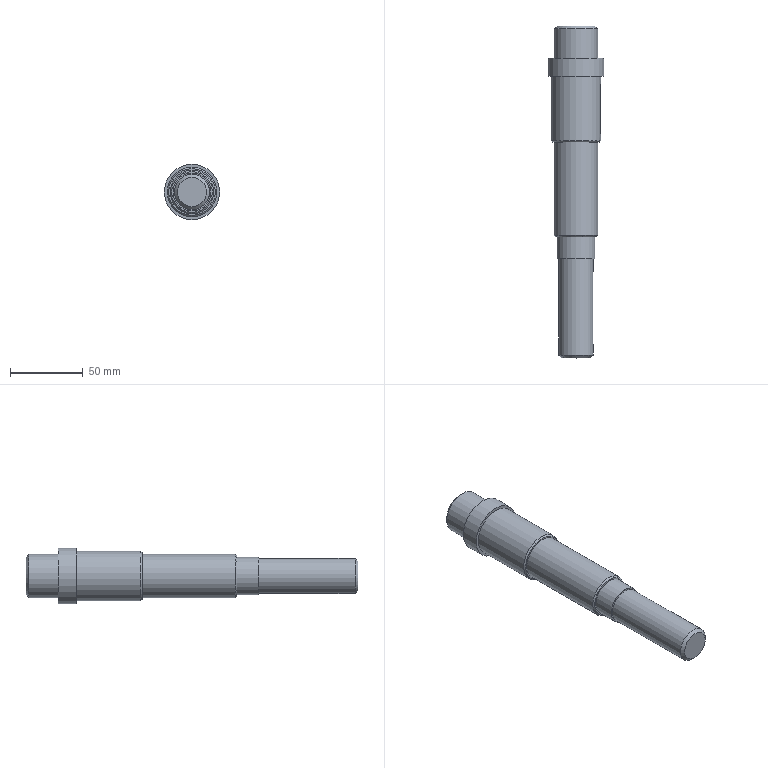Part | NX | features DATUM_CSYS 4, SKETCH 3, CHAMFER 2, DATUM_PLANE 2, EXTRUDE 2, CPROJ 1, SWP104 1 | 1 solid | 27 faces | box 38 x 227.5 x 38 mm | volume 152701 mm3 | plane 13 | cylinder 10 | cone 4 | commonest cylinder face diameters 6 x2 8 x2 30 x2 24 x1 26 x1 34 x1
STEP:
#1=CARTESIAN_POINT('',(0.,227.5,-13.));
#2=VERTEX_POINT('',#1);
#3=CARTESIAN_POINT('',(0.,227.5,0.));
#4=DIRECTION('',(0.,-1.,0.));
#5=DIRECTION('',(0.,0.,-1.));
#6=AXIS2_PLACEMENT_3D('',#3,#4,#5);
#7=CIRCLE('',#6,13.);
#8=EDGE_CURVE('',#2,#2,#7,.F.);
#9=ORIENTED_EDGE('',*,*,#8,.T.);
#10=EDGE_LOOP('',(#9));
#11=FACE_BOUND('',#10,.T.);
#12=CARTESIAN_POINT('',(0.,227.5,0.));
#13=DIRECTION('',(0.,-1.,0.));
#14=DIRECTION('',(0.,0.,-1.));
#15=AXIS2_PLACEMENT_3D('',#12,#13,#14);
#16=PLANE('',#15);
#17=ADVANCED_FACE('',(#11),#16,.F.);
#18=CARTESIAN_POINT('',(0.,225.5,-15.));
#19=VERTEX_POINT('',#18);
#20=CARTESIAN_POINT('',(0.,225.5,0.));
#21=DIRECTION('',(0.,-1.,0.));
#22=DIRECTION('',(0.,0.,-1.));
#23=AXIS2_PLACEMENT_3D('',#20,#21,#22);
#24=CIRCLE('',#23,15.);
#25=EDGE_CURVE('',#19,#19,#24,.T.);
#26=ORIENTED_EDGE('',*,*,#25,.T.);
#27=EDGE_LOOP('',(#26));
#28=FACE_BOUND('',#27,.T.);
#29=CARTESIAN_POINT('',(0.,205.5,-15.));
#30=VERTEX_POINT('',#29);
#31=CARTESIAN_POINT('',(0.,205.5,0.));
#32=DIRECTION('',(0.,-1.,0.));
#33=DIRECTION('',(0.,0.,-1.));
#34=AXIS2_PLACEMENT_3D('',#31,#32,#33);
#35=CIRCLE('',#34,15.);
#36=EDGE_CURVE('',#30,#30,#35,.T.);
#37=ORIENTED_EDGE('',*,*,#36,.F.);
#38=EDGE_LOOP('',(#37));
#39=FACE_BOUND('',#38,.T.);
#40=CARTESIAN_POINT('',(0.,227.5,0.));
#41=DIRECTION('',(0.,-1.,0.));
#42=DIRECTION('',(0.,0.,-1.));
#43=AXIS2_PLACEMENT_3D('',#40,#41,#42);
#44=CYLINDRICAL_SURFACE('',#43,15.);
#45=ADVANCED_FACE('',(#28,#39),#44,.T.);
#46=CARTESIAN_POINT('',(0.,205.5,-19.));
#47=VERTEX_POINT('',#46);
#48=CARTESIAN_POINT('',(0.,205.5,0.));
#49=DIRECTION('',(0.,-1.,0.));
#50=DIRECTION('',(0.,0.,-1.));
#51=AXIS2_PLACEMENT_3D('',#48,#49,#50);
#52=CIRCLE('',#51,19.);
#53=EDGE_CURVE('',#47,#47,#52,.T.);
#54=ORIENTED_EDGE('',*,*,#53,.F.);
#55=EDGE_LOOP('',(#54));
#56=FACE_BOUND('',#55,.T.);
#57=ORIENTED_EDGE('',*,*,#36,.T.);
#58=EDGE_LOOP('',(#57));
#59=FACE_BOUND('',#58,.T.);
#60=CARTESIAN_POINT('',(0.,205.5,15.));
#61=DIRECTION('',(0.,-1.,0.));
#62=DIRECTION('',(0.,0.,-1.));
#63=AXIS2_PLACEMENT_3D('',#60,#61,#62);
#64=PLANE('',#63);
#65=ADVANCED_FACE('',(#56,#59),#64,.F.);
#66=CARTESIAN_POINT('',(0.,193.,-19.));
#67=VERTEX_POINT('',#66);
#68=CARTESIAN_POINT('',(0.,193.,0.));
#69=DIRECTION('',(0.,-1.,0.));
#70=DIRECTION('',(0.,0.,-1.));
#71=AXIS2_PLACEMENT_3D('',#68,#69,#70);
#72=CIRCLE('',#71,19.);
#73=EDGE_CURVE('',#67,#67,#72,.T.);
#74=ORIENTED_EDGE('',*,*,#73,.F.);
#75=EDGE_LOOP('',(#74));
#76=FACE_BOUND('',#75,.T.);
#77=ORIENTED_EDGE('',*,*,#53,.T.);
#78=EDGE_LOOP('',(#77));
#79=FACE_BOUND('',#78,.T.);
#80=CARTESIAN_POINT('',(0.,227.5,0.));
#81=DIRECTION('',(0.,-1.,0.));
#82=DIRECTION('',(0.,0.,-1.));
#83=AXIS2_PLACEMENT_3D('',#80,#81,#82);
#84=CYLINDRICAL_SURFACE('',#83,19.);
#85=ADVANCED_FACE('',(#76,#79),#84,.T.);
#86=CARTESIAN_POINT('',(0.,193.,-17.));
#87=VERTEX_POINT('',#86);
#88=CARTESIAN_POINT('',(0.,193.,0.));
#89=DIRECTION('',(0.,-1.,0.));
#90=DIRECTION('',(0.,0.,-1.));
#91=AXIS2_PLACEMENT_3D('',#88,#89,#90);
#92=CIRCLE('',#91,17.);
#93=EDGE_CURVE('',#87,#87,#92,.T.);
#94=ORIENTED_EDGE('',*,*,#93,.F.);
#95=EDGE_LOOP('',(#94));
#96=FACE_BOUND('',#95,.T.);
#97=ORIENTED_EDGE('',*,*,#73,.T.);
#98=EDGE_LOOP('',(#97));
#99=FACE_BOUND('',#98,.T.);
#100=CARTESIAN_POINT('',(0.,193.,19.));
#101=DIRECTION('',(0.,1.,0.));
#102=DIRECTION('',(0.,0.,1.));
#103=AXIS2_PLACEMENT_3D('',#100,#101,#102);
#104=PLANE('',#103);
#105=ADVANCED_FACE('',(#96,#99),#104,.F.);
#106=CARTESIAN_POINT('',(16.523,156.5,4.));
#107=VERTEX_POINT('',#106);
#108=CARTESIAN_POINT('',(16.523,184.5,4.));
#109=VERTEX_POINT('',#108);
#110=CARTESIAN_POINT('',(16.523,227.5,4.));
#111=DIRECTION('',(0.,-1.,0.));
#112=VECTOR('',#111,1000.);
#113=LINE('',#110,#112);
#114=EDGE_CURVE('',#107,#109,#113,.F.);
#115=ORIENTED_EDGE('',*,*,#114,.T.);
#116=CARTESIAN_POINT('',(16.523,184.5,-4.));
#117=VERTEX_POINT('',#116);
#118=CARTESIAN_POINT('',(16.523,184.5,4.));
#119=CARTESIAN_POINT('',(16.523,185.561,4.));
#120=CARTESIAN_POINT('',(16.765,187.627,3.133));
#121=CARTESIAN_POINT('',(17.118,188.936,0.005404));
#122=CARTESIAN_POINT('',(16.765,187.629,-3.134));
#123=CARTESIAN_POINT('',(16.523,185.561,-4.));
#124=CARTESIAN_POINT('',(16.523,184.5,-4.));
#125=B_SPLINE_CURVE_WITH_KNOTS('',3,(#118,#119,#120,#121,#122,#123,#124),.UNSPECIFIED.,.F.,.F.,(4,1,1,1,4),(0.,0.003137,0.006273,0.00941,0.01255),.UNSPECIFIED.);
#126=EDGE_CURVE('',#109,#117,#125,.T.);
#127=ORIENTED_EDGE('',*,*,#126,.T.);
#128=CARTESIAN_POINT('',(16.523,156.5,-4.));
#129=VERTEX_POINT('',#128);
#130=CARTESIAN_POINT('',(16.523,227.5,-4.));
#131=DIRECTION('',(0.,-1.,0.));
#132=VECTOR('',#131,1000.);
#133=LINE('',#130,#132);
#134=EDGE_CURVE('',#117,#129,#133,.T.);
#135=ORIENTED_EDGE('',*,*,#134,.T.);
#136=CARTESIAN_POINT('',(16.523,156.5,-4.));
#137=CARTESIAN_POINT('',(16.523,155.439,-4.));
#138=CARTESIAN_POINT('',(16.765,153.373,-3.133));
#139=CARTESIAN_POINT('',(17.118,152.064,-0.005404));
#140=CARTESIAN_POINT('',(16.765,153.371,3.134));
#141=CARTESIAN_POINT('',(16.523,155.439,4.));
#142=CARTESIAN_POINT('',(16.523,156.5,4.));
#143=B_SPLINE_CURVE_WITH_KNOTS('',3,(#136,#137,#138,#139,#140,#141,#142),.UNSPECIFIED.,.F.,.F.,(4,1,1,1,4),(0.,0.003137,0.006273,0.00941,0.01255),.UNSPECIFIED.);
#144=EDGE_CURVE('',#129,#107,#143,.T.);
#145=ORIENTED_EDGE('',*,*,#144,.T.);
#146=EDGE_LOOP('',(#115,#127,#135,#145));
#147=FACE_BOUND('',#146,.T.);
#148=CARTESIAN_POINT('',(0.,149.,17.));
#149=VERTEX_POINT('',#148);
#150=CARTESIAN_POINT('',(0.,149.,0.));
#151=DIRECTION('',(0.,1.,0.));
#152=DIRECTION('',(0.,0.,1.));
#153=AXIS2_PLACEMENT_3D('',#150,#151,#152);
#154=CIRCLE('',#153,17.);
#155=EDGE_CURVE('',#149,#149,#154,.T.);
#156=ORIENTED_EDGE('',*,*,#155,.T.);
#157=EDGE_LOOP('',(#156));
#158=FACE_BOUND('',#157,.T.);
#159=ORIENTED_EDGE('',*,*,#93,.T.);
#160=EDGE_LOOP('',(#159));
#161=FACE_BOUND('',#160,.T.);
#162=CARTESIAN_POINT('',(0.,227.5,0.));
#163=DIRECTION('',(0.,-1.,0.));
#164=DIRECTION('',(0.,0.,-1.));
#165=AXIS2_PLACEMENT_3D('',#162,#163,#164);
#166=CYLINDRICAL_SURFACE('',#165,17.);
#167=ADVANCED_FACE('',(#147,#158,#161),#166,.T.);
#168=CARTESIAN_POINT('',(0.,148.,16.));
#169=VERTEX_POINT('',#168);
#170=CARTESIAN_POINT('',(0.,148.,0.));
#171=DIRECTION('',(0.,1.,0.));
#172=DIRECTION('',(0.,0.,1.));
#173=AXIS2_PLACEMENT_3D('',#170,#171,#172);
#174=CIRCLE('',#173,16.);
#175=EDGE_CURVE('',#169,#169,#174,.F.);
#176=ORIENTED_EDGE('',*,*,#175,.T.);
#177=EDGE_LOOP('',(#176));
#178=FACE_BOUND('',#177,.T.);
#179=CARTESIAN_POINT('',(0.,148.,-15.));
#180=VERTEX_POINT('',#179);
#181=CARTESIAN_POINT('',(0.,148.,0.));
#182=DIRECTION('',(0.,-1.,0.));
#183=DIRECTION('',(0.,0.,-1.));
#184=AXIS2_PLACEMENT_3D('',#181,#182,#183);
#185=CIRCLE('',#184,15.);
#186=EDGE_CURVE('',#180,#180,#185,.T.);
#187=ORIENTED_EDGE('',*,*,#186,.F.);
#188=EDGE_LOOP('',(#187));
#189=FACE_BOUND('',#188,.T.);
#190=CARTESIAN_POINT('',(0.,148.,17.));
#191=DIRECTION('',(0.,1.,0.));
#192=DIRECTION('',(0.,0.,1.));
#193=AXIS2_PLACEMENT_3D('',#190,#191,#192);
#194=PLANE('',#193);
#195=ADVANCED_FACE('',(#178,#189),#194,.F.);
#196=CARTESIAN_POINT('',(0.,84.,15.));
#197=VERTEX_POINT('',#196);
#198=CARTESIAN_POINT('',(0.,84.,0.));
#199=DIRECTION('',(0.,1.,0.));
#200=DIRECTION('',(0.,0.,1.));
#201=AXIS2_PLACEMENT_3D('',#198,#199,#200);
#202=CIRCLE('',#201,15.);
#203=EDGE_CURVE('',#197,#197,#202,.T.);
#204=ORIENTED_EDGE('',*,*,#203,.T.);
#205=EDGE_LOOP('',(#204));
#206=FACE_BOUND('',#205,.T.);
#207=ORIENTED_EDGE('',*,*,#186,.T.);
#208=EDGE_LOOP('',(#207));
#209=FACE_BOUND('',#208,.T.);
#210=CARTESIAN_POINT('',(0.,227.5,0.));
#211=DIRECTION('',(0.,-1.,0.));
#212=DIRECTION('',(0.,0.,-1.));
#213=AXIS2_PLACEMENT_3D('',#210,#211,#212);
#214=CYLINDRICAL_SURFACE('',#213,15.);
#215=ADVANCED_FACE('',(#206,#209),#214,.T.);
#216=CARTESIAN_POINT('',(0.,83.,14.));
#217=VERTEX_POINT('',#216);
#218=CARTESIAN_POINT('',(0.,83.,0.));
#219=DIRECTION('',(0.,1.,0.));
#220=DIRECTION('',(0.,0.,1.));
#221=AXIS2_PLACEMENT_3D('',#218,#219,#220);
#222=CIRCLE('',#221,14.);
#223=EDGE_CURVE('',#217,#217,#222,.F.);
#224=ORIENTED_EDGE('',*,*,#223,.T.);
#225=EDGE_LOOP('',(#224));
#226=FACE_BOUND('',#225,.T.);
#227=CARTESIAN_POINT('',(0.,83.,-13.));
#228=VERTEX_POINT('',#227);
#229=CARTESIAN_POINT('',(0.,83.,0.));
#230=DIRECTION('',(0.,-1.,0.));
#231=DIRECTION('',(0.,0.,-1.));
#232=AXIS2_PLACEMENT_3D('',#229,#230,#231);
#233=CIRCLE('',#232,13.);
#234=EDGE_CURVE('',#228,#228,#233,.T.);
#235=ORIENTED_EDGE('',*,*,#234,.F.);
#236=EDGE_LOOP('',(#235));
#237=FACE_BOUND('',#236,.T.);
#238=CARTESIAN_POINT('',(0.,83.,15.));
#239=DIRECTION('',(0.,1.,0.));
#240=DIRECTION('',(0.,0.,1.));
#241=AXIS2_PLACEMENT_3D('',#238,#239,#240);
#242=PLANE('',#241);
#243=ADVANCED_FACE('',(#226,#237),#242,.F.);
#244=CARTESIAN_POINT('',(0.,68.,-13.));
#245=VERTEX_POINT('',#244);
#246=CARTESIAN_POINT('',(0.,68.,0.));
#247=DIRECTION('',(0.,-1.,0.));
#248=DIRECTION('',(0.,0.,-1.));
#249=AXIS2_PLACEMENT_3D('',#246,#247,#248);
#250=CIRCLE('',#249,13.);
#251=EDGE_CURVE('',#245,#245,#250,.T.);
#252=ORIENTED_EDGE('',*,*,#251,.F.);
#253=EDGE_LOOP('',(#252));
#254=FACE_BOUND('',#253,.T.);
#255=ORIENTED_EDGE('',*,*,#234,.T.);
#256=EDGE_LOOP('',(#255));
#257=FACE_BOUND('',#256,.T.);
#258=CARTESIAN_POINT('',(0.,227.5,0.));
#259=DIRECTION('',(0.,-1.,0.));
#260=DIRECTION('',(0.,0.,-1.));
#261=AXIS2_PLACEMENT_3D('',#258,#259,#260);
#262=CYLINDRICAL_SURFACE('',#261,13.);
#263=ADVANCED_FACE('',(#254,#257),#262,.T.);
#264=CARTESIAN_POINT('',(0.,68.,-12.));
#265=VERTEX_POINT('',#264);
#266=CARTESIAN_POINT('',(0.,68.,0.));
#267=DIRECTION('',(0.,-1.,0.));
#268=DIRECTION('',(0.,0.,-1.));
#269=AXIS2_PLACEMENT_3D('',#266,#267,#268);
#270=CIRCLE('',#269,12.);
#271=EDGE_CURVE('',#265,#265,#270,.T.);
#272=ORIENTED_EDGE('',*,*,#271,.F.);
#273=EDGE_LOOP('',(#272));
#274=FACE_BOUND('',#273,.T.);
#275=ORIENTED_EDGE('',*,*,#251,.T.);
#276=EDGE_LOOP('',(#275));
#277=FACE_BOUND('',#276,.T.);
#278=CARTESIAN_POINT('',(0.,68.,13.));
#279=DIRECTION('',(0.,1.,0.));
#280=DIRECTION('',(0.,0.,1.));
#281=AXIS2_PLACEMENT_3D('',#278,#279,#280);
#282=PLANE('',#281);
#283=ADVANCED_FACE('',(#274,#277),#282,.F.);
#284=CARTESIAN_POINT('',(11.619,10.,3.));
#285=VERTEX_POINT('',#284);
#286=CARTESIAN_POINT('',(11.619,58.,3.));
#287=VERTEX_POINT('',#286);
#288=CARTESIAN_POINT('',(11.619,227.5,3.));
#289=DIRECTION('',(0.,-1.,0.));
#290=VECTOR('',#289,1000.);
#291=LINE('',#288,#290);
#292=EDGE_CURVE('',#285,#287,#291,.F.);
#293=ORIENTED_EDGE('',*,*,#292,.T.);
#294=CARTESIAN_POINT('',(11.619,58.,-3.));
#295=VERTEX_POINT('',#294);
#296=CARTESIAN_POINT('',(11.619,58.,3.));
#297=CARTESIAN_POINT('',(11.619,58.796,3.));
#298=CARTESIAN_POINT('',(11.813,60.345,2.35));
#299=CARTESIAN_POINT('',(12.094,61.327,0.004206));
#300=CARTESIAN_POINT('',(11.813,60.346,-2.35));
#301=CARTESIAN_POINT('',(11.619,58.796,-3.));
#302=CARTESIAN_POINT('',(11.619,58.,-3.));
#303=B_SPLINE_CURVE_WITH_KNOTS('',3,(#296,#297,#298,#299,#300,#301,#302),.UNSPECIFIED.,.F.,.F.,(4,1,1,1,4),(0.,0.002353,0.004707,0.00706,0.009414),.UNSPECIFIED.);
#304=EDGE_CURVE('',#287,#295,#303,.T.);
#305=ORIENTED_EDGE('',*,*,#304,.T.);
#306=CARTESIAN_POINT('',(11.619,10.,-3.));
#307=VERTEX_POINT('',#306);
#308=CARTESIAN_POINT('',(11.619,227.5,-3.));
#309=DIRECTION('',(0.,-1.,0.));
#310=VECTOR('',#309,1000.);
#311=LINE('',#308,#310);
#312=EDGE_CURVE('',#295,#307,#311,.T.);
#313=ORIENTED_EDGE('',*,*,#312,.T.);
#314=CARTESIAN_POINT('',(11.619,10.,-3.));
#315=CARTESIAN_POINT('',(11.619,9.204,-3.));
#316=CARTESIAN_POINT('',(11.813,7.655,-2.35));
#317=CARTESIAN_POINT('',(12.094,6.673,-0.004206));
#318=CARTESIAN_POINT('',(11.813,7.654,2.35));
#319=CARTESIAN_POINT('',(11.619,9.204,3.));
#320=CARTESIAN_POINT('',(11.619,10.,3.));
#321=B_SPLINE_CURVE_WITH_KNOTS('',3,(#314,#315,#316,#317,#318,#319,#320),.UNSPECIFIED.,.F.,.F.,(4,1,1,1,4),(0.,0.002353,0.004707,0.00706,0.009414),.UNSPECIFIED.);
#322=EDGE_CURVE('',#307,#285,#321,.T.);
#323=ORIENTED_EDGE('',*,*,#322,.T.);
#324=EDGE_LOOP('',(#293,#305,#313,#323));
#325=FACE_BOUND('',#324,.T.);
#326=CARTESIAN_POINT('',(0.,2.,12.));
#327=VERTEX_POINT('',#326);
#328=CARTESIAN_POINT('',(0.,2.,0.));
#329=DIRECTION('',(0.,1.,0.));
#330=DIRECTION('',(0.,0.,1.));
#331=AXIS2_PLACEMENT_3D('',#328,#329,#330);
#332=CIRCLE('',#331,12.);
#333=EDGE_CURVE('',#327,#327,#332,.T.);
#334=ORIENTED_EDGE('',*,*,#333,.T.);
#335=EDGE_LOOP('',(#334));
#336=FACE_BOUND('',#335,.T.);
#337=ORIENTED_EDGE('',*,*,#271,.T.);
#338=EDGE_LOOP('',(#337));
#339=FACE_BOUND('',#338,.T.);
#340=CARTESIAN_POINT('',(0.,227.5,0.));
#341=DIRECTION('',(0.,-1.,0.));
#342=DIRECTION('',(0.,0.,-1.));
#343=AXIS2_PLACEMENT_3D('',#340,#341,#342);
#344=CYLINDRICAL_SURFACE('',#343,12.);
#345=ADVANCED_FACE('',(#325,#336,#339),#344,.T.);
#346=CARTESIAN_POINT('',(0.,0.,10.));
#347=VERTEX_POINT('',#346);
#348=CARTESIAN_POINT('',(0.,0.,0.));
#349=DIRECTION('',(0.,1.,0.));
#350=DIRECTION('',(0.,0.,1.));
#351=AXIS2_PLACEMENT_3D('',#348,#349,#350);
#352=CIRCLE('',#351,10.);
#353=EDGE_CURVE('',#347,#347,#352,.F.);
#354=ORIENTED_EDGE('',*,*,#353,.T.);
#355=EDGE_LOOP('',(#354));
#356=FACE_BOUND('',#355,.T.);
#357=CARTESIAN_POINT('',(0.,0.,12.));
#358=DIRECTION('',(0.,1.,0.));
#359=DIRECTION('',(0.,0.,1.));
#360=AXIS2_PLACEMENT_3D('',#357,#358,#359);
#361=PLANE('',#360);
#362=ADVANCED_FACE('',(#356),#361,.F.);
#363=ORIENTED_EDGE('',*,*,#333,.F.);
#364=EDGE_LOOP('',(#363));
#365=FACE_BOUND('',#364,.T.);
#366=ORIENTED_EDGE('',*,*,#353,.F.);
#367=EDGE_LOOP('',(#366));
#368=FACE_BOUND('',#367,.T.);
#369=CARTESIAN_POINT('',(0.,0.,0.));
#370=DIRECTION('',(0.,1.,0.));
#371=DIRECTION('',(0.,0.,1.));
#372=AXIS2_PLACEMENT_3D('',#369,#370,#371);
#373=CONICAL_SURFACE('',#372,10.,0.7854);
#374=ADVANCED_FACE('',(#365,#368),#373,.T.);
#375=ORIENTED_EDGE('',*,*,#8,.F.);
#376=EDGE_LOOP('',(#375));
#377=FACE_BOUND('',#376,.T.);
#378=ORIENTED_EDGE('',*,*,#25,.F.);
#379=EDGE_LOOP('',(#378));
#380=FACE_BOUND('',#379,.T.);
#381=CARTESIAN_POINT('',(0.,225.5,0.));
#382=DIRECTION('',(0.,-1.,0.));
#383=DIRECTION('',(0.,0.,-1.));
#384=AXIS2_PLACEMENT_3D('',#381,#382,#383);
#385=CONICAL_SURFACE('',#384,15.,0.7854);
#386=ADVANCED_FACE('',(#377,#380),#385,.T.);
#387=ORIENTED_EDGE('',*,*,#203,.F.);
#388=EDGE_LOOP('',(#387));
#389=FACE_BOUND('',#388,.T.);
#390=ORIENTED_EDGE('',*,*,#223,.F.);
#391=EDGE_LOOP('',(#390));
#392=FACE_BOUND('',#391,.T.);
#393=CARTESIAN_POINT('',(0.,83.,0.));
#394=DIRECTION('',(0.,1.,0.));
#395=DIRECTION('',(0.,0.,1.));
#396=AXIS2_PLACEMENT_3D('',#393,#394,#395);
#397=CONICAL_SURFACE('',#396,14.,0.7854);
#398=ADVANCED_FACE('',(#389,#392),#397,.T.);
#399=ORIENTED_EDGE('',*,*,#155,.F.);
#400=EDGE_LOOP('',(#399));
#401=FACE_BOUND('',#400,.T.);
#402=ORIENTED_EDGE('',*,*,#175,.F.);
#403=EDGE_LOOP('',(#402));
#404=FACE_BOUND('',#403,.T.);
#405=CARTESIAN_POINT('',(0.,148.,0.));
#406=DIRECTION('',(0.,1.,0.));
#407=DIRECTION('',(0.,0.,1.));
#408=AXIS2_PLACEMENT_3D('',#405,#406,#407);
#409=CONICAL_SURFACE('',#408,16.,0.7854);
#410=ADVANCED_FACE('',(#401,#404),#409,.T.);
#411=CARTESIAN_POINT('',(12.5,156.5,-4.));
#412=VERTEX_POINT('',#411);
#413=CARTESIAN_POINT('',(12.5,156.5,-4.));
#414=DIRECTION('',(1.,0.,0.));
#415=VECTOR('',#414,1000.);
#416=LINE('',#413,#415);
#417=EDGE_CURVE('',#129,#412,#416,.F.);
#418=ORIENTED_EDGE('',*,*,#417,.T.);
#419=CARTESIAN_POINT('',(12.5,156.5,4.));
#420=VERTEX_POINT('',#419);
#421=CARTESIAN_POINT('',(12.5,156.5,0.));
#422=DIRECTION('',(1.,0.,0.));
#423=DIRECTION('',(0.,1.,0.));
#424=AXIS2_PLACEMENT_3D('',#421,#422,#423);
#425=CIRCLE('',#424,4.);
#426=EDGE_CURVE('',#412,#420,#425,.F.);
#427=ORIENTED_EDGE('',*,*,#426,.T.);
#428=CARTESIAN_POINT('',(12.5,156.5,4.));
#429=DIRECTION('',(1.,0.,0.));
#430=VECTOR('',#429,1000.);
#431=LINE('',#428,#430);
#432=EDGE_CURVE('',#107,#420,#431,.F.);
#433=ORIENTED_EDGE('',*,*,#432,.F.);
#434=ORIENTED_EDGE('',*,*,#144,.F.);
#435=EDGE_LOOP('',(#418,#427,#433,#434));
#436=FACE_BOUND('',#435,.T.);
#437=CARTESIAN_POINT('',(12.5,156.5,0.));
#438=DIRECTION('',(1.,0.,0.));
#439=DIRECTION('',(0.,0.,-1.));
#440=AXIS2_PLACEMENT_3D('',#437,#438,#439);
#441=CYLINDRICAL_SURFACE('',#440,4.);
#442=ADVANCED_FACE('',(#436),#441,.F.);
#443=CARTESIAN_POINT('',(12.5,184.5,-4.));
#444=VERTEX_POINT('',#443);
#445=CARTESIAN_POINT('',(12.5,184.5,-4.));
#446=DIRECTION('',(1.,0.,0.));
#447=VECTOR('',#446,1000.);
#448=LINE('',#445,#447);
#449=EDGE_CURVE('',#117,#444,#448,.F.);
#450=ORIENTED_EDGE('',*,*,#449,.T.);
#451=CARTESIAN_POINT('',(12.5,156.5,-4.));
#452=DIRECTION('',(0.,1.,0.));
#453=VECTOR('',#452,1000.);
#454=LINE('',#451,#453);
#455=EDGE_CURVE('',#444,#412,#454,.F.);
#456=ORIENTED_EDGE('',*,*,#455,.T.);
#457=ORIENTED_EDGE('',*,*,#417,.F.);
#458=ORIENTED_EDGE('',*,*,#134,.F.);
#459=EDGE_LOOP('',(#450,#456,#457,#458));
#460=FACE_BOUND('',#459,.T.);
#461=CARTESIAN_POINT('',(12.5,156.5,-4.));
#462=DIRECTION('',(0.,0.,-1.));
#463=DIRECTION('',(0.,1.,0.));
#464=AXIS2_PLACEMENT_3D('',#461,#462,#463);
#465=PLANE('',#464);
#466=ADVANCED_FACE('',(#460),#465,.F.);
#467=CARTESIAN_POINT('',(12.5,184.5,4.));
#468=VERTEX_POINT('',#467);
#469=CARTESIAN_POINT('',(12.5,184.5,4.));
#470=DIRECTION('',(1.,0.,0.));
#471=VECTOR('',#470,1000.);
#472=LINE('',#469,#471);
#473=EDGE_CURVE('',#109,#468,#472,.F.);
#474=ORIENTED_EDGE('',*,*,#473,.T.);
#475=CARTESIAN_POINT('',(12.5,184.5,0.));
#476=DIRECTION('',(1.,0.,0.));
#477=DIRECTION('',(0.,1.,0.));
#478=AXIS2_PLACEMENT_3D('',#475,#476,#477);
#479=CIRCLE('',#478,4.);
#480=EDGE_CURVE('',#468,#444,#479,.F.);
#481=ORIENTED_EDGE('',*,*,#480,.T.);
#482=ORIENTED_EDGE('',*,*,#449,.F.);
#483=ORIENTED_EDGE('',*,*,#126,.F.);
#484=EDGE_LOOP('',(#474,#481,#482,#483));
#485=FACE_BOUND('',#484,.T.);
#486=CARTESIAN_POINT('',(12.5,184.5,0.));
#487=DIRECTION('',(1.,0.,0.));
#488=DIRECTION('',(0.,0.,-1.));
#489=AXIS2_PLACEMENT_3D('',#486,#487,#488);
#490=CYLINDRICAL_SURFACE('',#489,4.);
#491=ADVANCED_FACE('',(#485),#490,.F.);
#492=ORIENTED_EDGE('',*,*,#432,.T.);
#493=CARTESIAN_POINT('',(12.5,184.5,4.));
#494=DIRECTION('',(0.,-1.,0.));
#495=VECTOR('',#494,1000.);
#496=LINE('',#493,#495);
#497=EDGE_CURVE('',#420,#468,#496,.F.);
#498=ORIENTED_EDGE('',*,*,#497,.T.);
#499=ORIENTED_EDGE('',*,*,#473,.F.);
#500=ORIENTED_EDGE('',*,*,#114,.F.);
#501=EDGE_LOOP('',(#492,#498,#499,#500));
#502=FACE_BOUND('',#501,.T.);
#503=CARTESIAN_POINT('',(12.5,184.5,4.));
#504=DIRECTION('',(0.,0.,1.));
#505=DIRECTION('',(0.,-1.,0.));
#506=AXIS2_PLACEMENT_3D('',#503,#504,#505);
#507=PLANE('',#506);
#508=ADVANCED_FACE('',(#502),#507,.F.);
#509=ORIENTED_EDGE('',*,*,#426,.F.);
#510=ORIENTED_EDGE('',*,*,#455,.F.);
#511=ORIENTED_EDGE('',*,*,#480,.F.);
#512=ORIENTED_EDGE('',*,*,#497,.F.);
#513=EDGE_LOOP('',(#509,#510,#511,#512));
#514=FACE_BOUND('',#513,.T.);
#515=CARTESIAN_POINT('',(12.5,156.5,0.));
#516=DIRECTION('',(1.,0.,0.));
#517=DIRECTION('',(0.,0.,-1.));
#518=AXIS2_PLACEMENT_3D('',#515,#516,#517);
#519=PLANE('',#518);
#520=ADVANCED_FACE('',(#514),#519,.T.);
#521=CARTESIAN_POINT('',(8.9,10.,-3.));
#522=VERTEX_POINT('',#521);
#523=CARTESIAN_POINT('',(8.9,10.,-3.));
#524=DIRECTION('',(1.,0.,0.));
#525=VECTOR('',#524,1000.);
#526=LINE('',#523,#525);
#527=EDGE_CURVE('',#307,#522,#526,.F.);
#528=ORIENTED_EDGE('',*,*,#527,.T.);
#529=CARTESIAN_POINT('',(8.9,10.,3.));
#530=VERTEX_POINT('',#529);
#531=CARTESIAN_POINT('',(8.9,10.,0.));
#532=DIRECTION('',(1.,0.,0.));
#533=DIRECTION('',(0.,1.,0.));
#534=AXIS2_PLACEMENT_3D('',#531,#532,#533);
#535=CIRCLE('',#534,3.);
#536=EDGE_CURVE('',#522,#530,#535,.F.);
#537=ORIENTED_EDGE('',*,*,#536,.T.);
#538=CARTESIAN_POINT('',(8.9,10.,3.));
#539=DIRECTION('',(1.,0.,0.));
#540=VECTOR('',#539,1000.);
#541=LINE('',#538,#540);
#542=EDGE_CURVE('',#285,#530,#541,.F.);
#543=ORIENTED_EDGE('',*,*,#542,.F.);
#544=ORIENTED_EDGE('',*,*,#322,.F.);
#545=EDGE_LOOP('',(#528,#537,#543,#544));
#546=FACE_BOUND('',#545,.T.);
#547=CARTESIAN_POINT('',(8.9,10.,0.));
#548=DIRECTION('',(1.,0.,0.));
#549=DIRECTION('',(0.,0.,-1.));
#550=AXIS2_PLACEMENT_3D('',#547,#548,#549);
#551=CYLINDRICAL_SURFACE('',#550,3.);
#552=ADVANCED_FACE('',(#546),#551,.F.);
#553=CARTESIAN_POINT('',(8.9,58.,-3.));
#554=VERTEX_POINT('',#553);
#555=CARTESIAN_POINT('',(8.9,58.,-3.));
#556=DIRECTION('',(1.,0.,0.));
#557=VECTOR('',#556,1000.);
#558=LINE('',#555,#557);
#559=EDGE_CURVE('',#295,#554,#558,.F.);
#560=ORIENTED_EDGE('',*,*,#559,.T.);
#561=CARTESIAN_POINT('',(8.9,10.,-3.));
#562=DIRECTION('',(0.,1.,0.));
#563=VECTOR('',#562,1000.);
#564=LINE('',#561,#563);
#565=EDGE_CURVE('',#554,#522,#564,.F.);
#566=ORIENTED_EDGE('',*,*,#565,.T.);
#567=ORIENTED_EDGE('',*,*,#527,.F.);
#568=ORIENTED_EDGE('',*,*,#312,.F.);
#569=EDGE_LOOP('',(#560,#566,#567,#568));
#570=FACE_BOUND('',#569,.T.);
#571=CARTESIAN_POINT('',(8.9,10.,-3.));
#572=DIRECTION('',(0.,0.,-1.));
#573=DIRECTION('',(0.,1.,0.));
#574=AXIS2_PLACEMENT_3D('',#571,#572,#573);
#575=PLANE('',#574);
#576=ADVANCED_FACE('',(#570),#575,.F.);
#577=CARTESIAN_POINT('',(8.9,58.,3.));
#578=VERTEX_POINT('',#577);
#579=CARTESIAN_POINT('',(8.9,58.,3.));
#580=DIRECTION('',(1.,0.,0.));
#581=VECTOR('',#580,1000.);
#582=LINE('',#579,#581);
#583=EDGE_CURVE('',#287,#578,#582,.F.);
#584=ORIENTED_EDGE('',*,*,#583,.T.);
#585=CARTESIAN_POINT('',(8.9,58.,0.));
#586=DIRECTION('',(1.,0.,0.));
#587=DIRECTION('',(0.,1.,0.));
#588=AXIS2_PLACEMENT_3D('',#585,#586,#587);
#589=CIRCLE('',#588,3.);
#590=EDGE_CURVE('',#578,#554,#589,.F.);
#591=ORIENTED_EDGE('',*,*,#590,.T.);
#592=ORIENTED_EDGE('',*,*,#559,.F.);
#593=ORIENTED_EDGE('',*,*,#304,.F.);
#594=EDGE_LOOP('',(#584,#591,#592,#593));
#595=FACE_BOUND('',#594,.T.);
#596=CARTESIAN_POINT('',(8.9,58.,0.));
#597=DIRECTION('',(1.,0.,0.));
#598=DIRECTION('',(0.,0.,-1.));
#599=AXIS2_PLACEMENT_3D('',#596,#597,#598);
#600=CYLINDRICAL_SURFACE('',#599,3.);
#601=ADVANCED_FACE('',(#595),#600,.F.);
#602=ORIENTED_EDGE('',*,*,#542,.T.);
#603=CARTESIAN_POINT('',(8.9,58.,3.));
#604=DIRECTION('',(0.,-1.,0.));
#605=VECTOR('',#604,1000.);
#606=LINE('',#603,#605);
#607=EDGE_CURVE('',#530,#578,#606,.F.);
#608=ORIENTED_EDGE('',*,*,#607,.T.);
#609=ORIENTED_EDGE('',*,*,#583,.F.);
#610=ORIENTED_EDGE('',*,*,#292,.F.);
#611=EDGE_LOOP('',(#602,#608,#609,#610));
#612=FACE_BOUND('',#611,.T.);
#613=CARTESIAN_POINT('',(8.9,58.,3.));
#614=DIRECTION('',(0.,0.,1.));
#615=DIRECTION('',(0.,-1.,0.));
#616=AXIS2_PLACEMENT_3D('',#613,#614,#615);
#617=PLANE('',#616);
#618=ADVANCED_FACE('',(#612),#617,.F.);
#619=ORIENTED_EDGE('',*,*,#536,.F.);
#620=ORIENTED_EDGE('',*,*,#565,.F.);
#621=ORIENTED_EDGE('',*,*,#590,.F.);
#622=ORIENTED_EDGE('',*,*,#607,.F.);
#623=EDGE_LOOP('',(#619,#620,#621,#622));
#624=FACE_BOUND('',#623,.T.);
#625=CARTESIAN_POINT('',(8.9,10.,0.));
#626=DIRECTION('',(1.,0.,0.));
#627=DIRECTION('',(0.,0.,-1.));
#628=AXIS2_PLACEMENT_3D('',#625,#626,#627);
#629=PLANE('',#628);
#630=ADVANCED_FACE('',(#624),#629,.T.);
#631=CLOSED_SHELL('',(#17,#45,#65,#85,#105,#167,#195,#215,#243,#263,#283,#345,#362,#374,#386,#398,#410,#442,#466,#491,#508,#520,#552,#576,#601,#618,#630));
#632=MANIFOLD_SOLID_BREP('',#631);
#633=(LENGTH_UNIT()NAMED_UNIT(*)SI_UNIT(.MILLI.,.METRE.));
#634=UNCERTAINTY_MEASURE_WITH_UNIT(LENGTH_MEASURE(0.0508),#633,'','');
#635=(NAMED_UNIT(*)PLANE_ANGLE_UNIT()SI_UNIT($,.RADIAN.));
#636=(NAMED_UNIT(*)SI_UNIT($,.STERADIAN.)SOLID_ANGLE_UNIT());
#637=(GEOMETRIC_REPRESENTATION_CONTEXT(3)GLOBAL_UNCERTAINTY_ASSIGNED_CONTEXT((#634))GLOBAL_UNIT_ASSIGNED_CONTEXT((#633,#635,#636))REPRESENTATION_CONTEXT('',''));
#638=ADVANCED_BREP_SHAPE_REPRESENTATION('',(#632),#637);